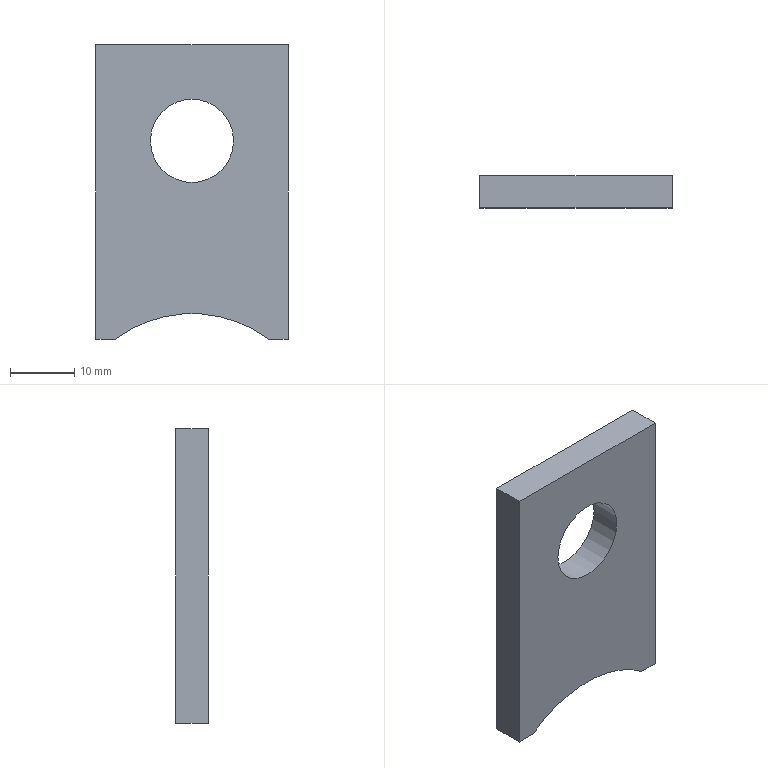Part | NX | features solid 2 | 1 solid | 9 faces | box 30 x 5 x 46 mm | volume 5909 mm3 | plane 7 | cylinder 2 | commonest cylinder face diameters 13 x1 40 x1
STEP:
#1=CARTESIAN_POINT('',(-688.,-535.,192.));
#2=VERTEX_POINT('',#1);
#3=CARTESIAN_POINT('',(-685.,-535.,192.));
#4=VERTEX_POINT('',#3);
#5=CARTESIAN_POINT('',(-688.,-535.,192.));
#6=DIRECTION('',(1.,0.,0.));
#7=VECTOR('',#6,1000.);
#8=LINE('',#5,#7);
#9=EDGE_CURVE('',#2,#4,#8,.T.);
#10=ORIENTED_EDGE('',*,*,#9,.T.);
#11=CARTESIAN_POINT('',(-685.,-540.,192.));
#12=VERTEX_POINT('',#11);
#13=CARTESIAN_POINT('',(-685.,-540.,192.));
#14=DIRECTION('',(0.,1.,0.));
#15=VECTOR('',#14,1000.);
#16=LINE('',#13,#15);
#17=EDGE_CURVE('',#12,#4,#16,.T.);
#18=ORIENTED_EDGE('',*,*,#17,.F.);
#19=CARTESIAN_POINT('',(-688.,-540.,192.));
#20=VERTEX_POINT('',#19);
#21=CARTESIAN_POINT('',(-688.,-540.,192.));
#22=DIRECTION('',(1.,0.,0.));
#23=VECTOR('',#22,1000.);
#24=LINE('',#21,#23);
#25=EDGE_CURVE('',#20,#12,#24,.T.);
#26=ORIENTED_EDGE('',*,*,#25,.F.);
#27=CARTESIAN_POINT('',(-688.,-540.,192.));
#28=DIRECTION('',(0.,1.,0.));
#29=VECTOR('',#28,1000.);
#30=LINE('',#27,#29);
#31=EDGE_CURVE('',#20,#2,#30,.T.);
#32=ORIENTED_EDGE('',*,*,#31,.T.);
#33=EDGE_LOOP('',(#10,#18,#26,#32));
#34=FACE_BOUND('',#33,.T.);
#35=CARTESIAN_POINT('',(-688.,-540.,192.));
#36=DIRECTION('',(0.,0.,-1.));
#37=DIRECTION('',(1.,0.,0.));
#38=AXIS2_PLACEMENT_3D('',#35,#36,#37);
#39=PLANE('',#38);
#40=ADVANCED_FACE('',(#34),#39,.T.);
#41=CARTESIAN_POINT('',(-685.,-535.,238.));
#42=VERTEX_POINT('',#41);
#43=CARTESIAN_POINT('',(-685.,-535.,192.));
#44=DIRECTION('',(0.,0.,1.));
#45=VECTOR('',#44,1000.);
#46=LINE('',#43,#45);
#47=EDGE_CURVE('',#4,#42,#46,.T.);
#48=ORIENTED_EDGE('',*,*,#47,.T.);
#49=CARTESIAN_POINT('',(-685.,-540.,238.));
#50=VERTEX_POINT('',#49);
#51=CARTESIAN_POINT('',(-685.,-540.,238.));
#52=DIRECTION('',(0.,1.,0.));
#53=VECTOR('',#52,1000.);
#54=LINE('',#51,#53);
#55=EDGE_CURVE('',#50,#42,#54,.T.);
#56=ORIENTED_EDGE('',*,*,#55,.F.);
#57=CARTESIAN_POINT('',(-685.,-540.,192.));
#58=DIRECTION('',(0.,0.,1.));
#59=VECTOR('',#58,1000.);
#60=LINE('',#57,#59);
#61=EDGE_CURVE('',#12,#50,#60,.T.);
#62=ORIENTED_EDGE('',*,*,#61,.F.);
#63=ORIENTED_EDGE('',*,*,#17,.T.);
#64=EDGE_LOOP('',(#48,#56,#62,#63));
#65=FACE_BOUND('',#64,.T.);
#66=CARTESIAN_POINT('',(-685.,-540.,192.));
#67=DIRECTION('',(1.,0.,0.));
#68=DIRECTION('',(0.,0.,1.));
#69=AXIS2_PLACEMENT_3D('',#66,#67,#68);
#70=PLANE('',#69);
#71=ADVANCED_FACE('',(#65),#70,.T.);
#72=CARTESIAN_POINT('',(-715.,-535.,238.));
#73=VERTEX_POINT('',#72);
#74=CARTESIAN_POINT('',(-685.,-535.,238.));
#75=DIRECTION('',(-1.,0.,0.));
#76=VECTOR('',#75,1000.);
#77=LINE('',#74,#76);
#78=EDGE_CURVE('',#42,#73,#77,.T.);
#79=ORIENTED_EDGE('',*,*,#78,.T.);
#80=CARTESIAN_POINT('',(-715.,-540.,238.));
#81=VERTEX_POINT('',#80);
#82=CARTESIAN_POINT('',(-715.,-540.,238.));
#83=DIRECTION('',(0.,1.,0.));
#84=VECTOR('',#83,1000.);
#85=LINE('',#82,#84);
#86=EDGE_CURVE('',#81,#73,#85,.T.);
#87=ORIENTED_EDGE('',*,*,#86,.F.);
#88=CARTESIAN_POINT('',(-685.,-540.,238.));
#89=DIRECTION('',(-1.,0.,0.));
#90=VECTOR('',#89,1000.);
#91=LINE('',#88,#90);
#92=EDGE_CURVE('',#50,#81,#91,.T.);
#93=ORIENTED_EDGE('',*,*,#92,.F.);
#94=ORIENTED_EDGE('',*,*,#55,.T.);
#95=EDGE_LOOP('',(#79,#87,#93,#94));
#96=FACE_BOUND('',#95,.T.);
#97=CARTESIAN_POINT('',(-685.,-540.,238.));
#98=DIRECTION('',(0.,0.,1.));
#99=DIRECTION('',(-1.,0.,0.));
#100=AXIS2_PLACEMENT_3D('',#97,#98,#99);
#101=PLANE('',#100);
#102=ADVANCED_FACE('',(#96),#101,.T.);
#103=CARTESIAN_POINT('',(-715.,-535.,192.));
#104=VERTEX_POINT('',#103);
#105=CARTESIAN_POINT('',(-715.,-535.,238.));
#106=DIRECTION('',(0.,0.,-1.));
#107=VECTOR('',#106,1000.);
#108=LINE('',#105,#107);
#109=EDGE_CURVE('',#73,#104,#108,.T.);
#110=ORIENTED_EDGE('',*,*,#109,.T.);
#111=CARTESIAN_POINT('',(-715.,-540.,192.));
#112=VERTEX_POINT('',#111);
#113=CARTESIAN_POINT('',(-715.,-540.,192.));
#114=DIRECTION('',(0.,1.,0.));
#115=VECTOR('',#114,1000.);
#116=LINE('',#113,#115);
#117=EDGE_CURVE('',#112,#104,#116,.T.);
#118=ORIENTED_EDGE('',*,*,#117,.F.);
#119=CARTESIAN_POINT('',(-715.,-540.,238.));
#120=DIRECTION('',(0.,0.,-1.));
#121=VECTOR('',#120,1000.);
#122=LINE('',#119,#121);
#123=EDGE_CURVE('',#81,#112,#122,.T.);
#124=ORIENTED_EDGE('',*,*,#123,.F.);
#125=ORIENTED_EDGE('',*,*,#86,.T.);
#126=EDGE_LOOP('',(#110,#118,#124,#125));
#127=FACE_BOUND('',#126,.T.);
#128=CARTESIAN_POINT('',(-715.,-540.,238.));
#129=DIRECTION('',(-1.,0.,0.));
#130=DIRECTION('',(0.,0.,-1.));
#131=AXIS2_PLACEMENT_3D('',#128,#129,#130);
#132=PLANE('',#131);
#133=ADVANCED_FACE('',(#127),#132,.T.);
#134=CARTESIAN_POINT('',(-712.,-535.,192.));
#135=VERTEX_POINT('',#134);
#136=CARTESIAN_POINT('',(-715.,-535.,192.));
#137=DIRECTION('',(1.,0.,0.));
#138=VECTOR('',#137,1000.);
#139=LINE('',#136,#138);
#140=EDGE_CURVE('',#104,#135,#139,.T.);
#141=ORIENTED_EDGE('',*,*,#140,.T.);
#142=CARTESIAN_POINT('',(-712.,-540.,192.));
#143=VERTEX_POINT('',#142);
#144=CARTESIAN_POINT('',(-712.,-540.,192.));
#145=DIRECTION('',(0.,1.,0.));
#146=VECTOR('',#145,1000.);
#147=LINE('',#144,#146);
#148=EDGE_CURVE('',#143,#135,#147,.T.);
#149=ORIENTED_EDGE('',*,*,#148,.F.);
#150=CARTESIAN_POINT('',(-715.,-540.,192.));
#151=DIRECTION('',(1.,0.,0.));
#152=VECTOR('',#151,1000.);
#153=LINE('',#150,#152);
#154=EDGE_CURVE('',#112,#143,#153,.T.);
#155=ORIENTED_EDGE('',*,*,#154,.F.);
#156=ORIENTED_EDGE('',*,*,#117,.T.);
#157=EDGE_LOOP('',(#141,#149,#155,#156));
#158=FACE_BOUND('',#157,.T.);
#159=CARTESIAN_POINT('',(-715.,-540.,192.));
#160=DIRECTION('',(0.,0.,-1.));
#161=DIRECTION('',(1.,0.,0.));
#162=AXIS2_PLACEMENT_3D('',#159,#160,#161);
#163=PLANE('',#162);
#164=ADVANCED_FACE('',(#158),#163,.T.);
#165=CARTESIAN_POINT('',(-700.,-535.,176.));
#166=DIRECTION('',(0.,1.,0.));
#167=DIRECTION('',(-1.,0.,0.));
#168=AXIS2_PLACEMENT_3D('',#165,#166,#167);
#169=CIRCLE('',#168,20.);
#170=EDGE_CURVE('',#135,#2,#169,.T.);
#171=ORIENTED_EDGE('',*,*,#170,.T.);
#172=ORIENTED_EDGE('',*,*,#31,.F.);
#173=CARTESIAN_POINT('',(-700.,-540.,176.));
#174=DIRECTION('',(0.,1.,0.));
#175=DIRECTION('',(-1.,0.,0.));
#176=AXIS2_PLACEMENT_3D('',#173,#174,#175);
#177=CIRCLE('',#176,20.);
#178=EDGE_CURVE('',#143,#20,#177,.T.);
#179=ORIENTED_EDGE('',*,*,#178,.F.);
#180=ORIENTED_EDGE('',*,*,#148,.T.);
#181=EDGE_LOOP('',(#171,#172,#179,#180));
#182=FACE_BOUND('',#181,.T.);
#183=CARTESIAN_POINT('',(-700.,-540.,176.));
#184=DIRECTION('',(0.,1.,0.));
#185=DIRECTION('',(0.,0.,1.));
#186=AXIS2_PLACEMENT_3D('',#183,#184,#185);
#187=CYLINDRICAL_SURFACE('',#186,20.);
#188=ADVANCED_FACE('',(#182),#187,.F.);
#189=CARTESIAN_POINT('',(-706.5,-540.,223.));
#190=VERTEX_POINT('',#189);
#191=CARTESIAN_POINT('',(-700.,-540.,223.));
#192=DIRECTION('',(0.,1.,0.));
#193=DIRECTION('',(-1.,0.,0.));
#194=AXIS2_PLACEMENT_3D('',#191,#192,#193);
#195=CIRCLE('',#194,6.5);
#196=EDGE_CURVE('',#190,#190,#195,.T.);
#197=ORIENTED_EDGE('',*,*,#196,.F.);
#198=EDGE_LOOP('',(#197));
#199=FACE_BOUND('',#198,.T.);
#200=CARTESIAN_POINT('',(-706.5,-535.,223.));
#201=VERTEX_POINT('',#200);
#202=CARTESIAN_POINT('',(-700.,-535.,223.));
#203=DIRECTION('',(0.,1.,0.));
#204=DIRECTION('',(-1.,0.,0.));
#205=AXIS2_PLACEMENT_3D('',#202,#203,#204);
#206=CIRCLE('',#205,6.5);
#207=EDGE_CURVE('',#201,#201,#206,.T.);
#208=ORIENTED_EDGE('',*,*,#207,.T.);
#209=EDGE_LOOP('',(#208));
#210=FACE_BOUND('',#209,.T.);
#211=CARTESIAN_POINT('',(-700.,-540.,223.));
#212=DIRECTION('',(0.,1.,0.));
#213=DIRECTION('',(0.,0.,1.));
#214=AXIS2_PLACEMENT_3D('',#211,#212,#213);
#215=CYLINDRICAL_SURFACE('',#214,6.5);
#216=ADVANCED_FACE('',(#199,#210),#215,.F.);
#217=ORIENTED_EDGE('',*,*,#25,.T.);
#218=ORIENTED_EDGE('',*,*,#61,.T.);
#219=ORIENTED_EDGE('',*,*,#92,.T.);
#220=ORIENTED_EDGE('',*,*,#123,.T.);
#221=ORIENTED_EDGE('',*,*,#154,.T.);
#222=ORIENTED_EDGE('',*,*,#178,.T.);
#223=EDGE_LOOP('',(#217,#218,#219,#220,#221,#222));
#224=FACE_BOUND('',#223,.T.);
#225=ORIENTED_EDGE('',*,*,#196,.T.);
#226=EDGE_LOOP('',(#225));
#227=FACE_BOUND('',#226,.T.);
#228=CARTESIAN_POINT('',(-700.,-540.,176.));
#229=DIRECTION('',(0.,-1.,0.));
#230=DIRECTION('',(0.,0.,-1.));
#231=AXIS2_PLACEMENT_3D('',#228,#229,#230);
#232=PLANE('',#231);
#233=ADVANCED_FACE('',(#224,#227),#232,.T.);
#234=ORIENTED_EDGE('',*,*,#9,.F.);
#235=ORIENTED_EDGE('',*,*,#170,.F.);
#236=ORIENTED_EDGE('',*,*,#140,.F.);
#237=ORIENTED_EDGE('',*,*,#109,.F.);
#238=ORIENTED_EDGE('',*,*,#78,.F.);
#239=ORIENTED_EDGE('',*,*,#47,.F.);
#240=EDGE_LOOP('',(#234,#235,#236,#237,#238,#239));
#241=FACE_BOUND('',#240,.T.);
#242=ORIENTED_EDGE('',*,*,#207,.F.);
#243=EDGE_LOOP('',(#242));
#244=FACE_BOUND('',#243,.T.);
#245=CARTESIAN_POINT('',(-700.,-535.,176.));
#246=DIRECTION('',(0.,-1.,0.));
#247=DIRECTION('',(0.,0.,-1.));
#248=AXIS2_PLACEMENT_3D('',#245,#246,#247);
#249=PLANE('',#248);
#250=ADVANCED_FACE('',(#241,#244),#249,.F.);
#251=CLOSED_SHELL('',(#40,#71,#102,#133,#164,#188,#216,#233,#250));
#252=MANIFOLD_SOLID_BREP('',#251);
#253=(LENGTH_UNIT()NAMED_UNIT(*)SI_UNIT(.MILLI.,.METRE.));
#254=UNCERTAINTY_MEASURE_WITH_UNIT(LENGTH_MEASURE(0.00001),#253,'','');
#255=(NAMED_UNIT(*)PLANE_ANGLE_UNIT()SI_UNIT($,.RADIAN.));
#256=(NAMED_UNIT(*)SI_UNIT($,.STERADIAN.)SOLID_ANGLE_UNIT());
#257=(GEOMETRIC_REPRESENTATION_CONTEXT(3)GLOBAL_UNCERTAINTY_ASSIGNED_CONTEXT((#254))GLOBAL_UNIT_ASSIGNED_CONTEXT((#253,#255,#256))REPRESENTATION_CONTEXT('',''));
#258=ADVANCED_BREP_SHAPE_REPRESENTATION('',(#252),#257);